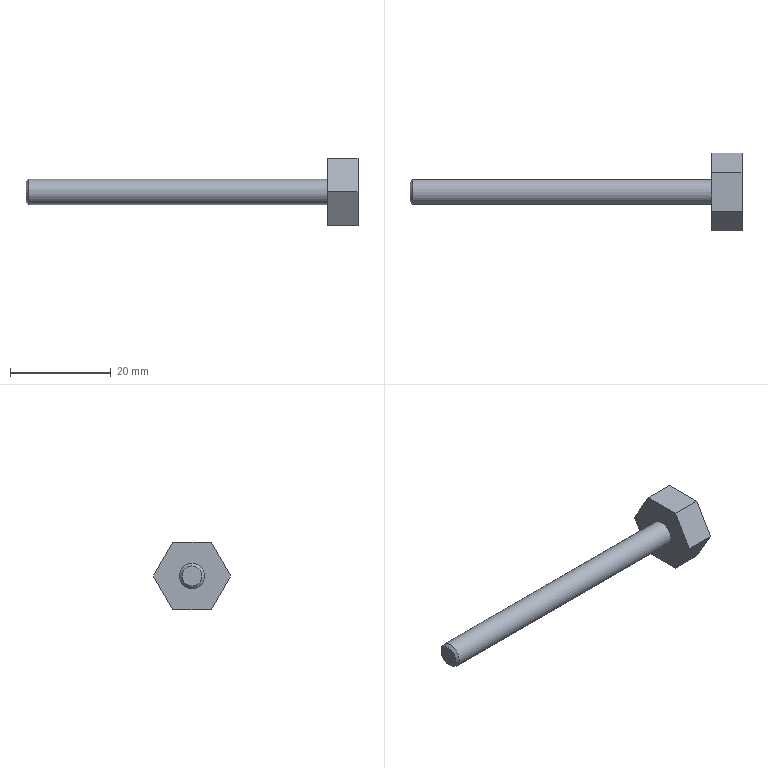Part | NX | features DATUM_CSYS 4, EXTRUDE 3, OFFSET_REGION 3, SKETCH 3, CHAMFER 1 | 1 solid | 18 faces | box 66 x 15.381 x 13.321 mm | volume 1888 mm3 | plane 16 | cylinder 1 | cone 1 | commonest cylinder face diameters 5 x1
STEP:
#1=CARTESIAN_POINT('',(76.,-7.691,0.));
#2=VERTEX_POINT('',#1);
#3=CARTESIAN_POINT('',(76.,-3.845,-6.66));
#4=VERTEX_POINT('',#3);
#5=CARTESIAN_POINT('',(76.,-8.268,1.));
#6=DIRECTION('',(0.,0.5,-0.866));
#7=VECTOR('',#6,1000.);
#8=LINE('',#5,#7);
#9=EDGE_CURVE('',#2,#4,#8,.T.);
#10=ORIENTED_EDGE('',*,*,#9,.T.);
#11=CARTESIAN_POINT('',(76.,3.845,-6.66));
#12=VERTEX_POINT('',#11);
#13=CARTESIAN_POINT('',(76.,-5.,-6.66));
#14=DIRECTION('',(0.,1.,0.));
#15=VECTOR('',#14,1000.);
#16=LINE('',#13,#15);
#17=EDGE_CURVE('',#4,#12,#16,.T.);
#18=ORIENTED_EDGE('',*,*,#17,.T.);
#19=CARTESIAN_POINT('',(76.,7.691,0.));
#20=VERTEX_POINT('',#19);
#21=CARTESIAN_POINT('',(76.,3.268,-7.66));
#22=DIRECTION('',(0.,0.5,0.866));
#23=VECTOR('',#22,1000.);
#24=LINE('',#21,#23);
#25=EDGE_CURVE('',#12,#20,#24,.T.);
#26=ORIENTED_EDGE('',*,*,#25,.T.);
#27=CARTESIAN_POINT('',(76.,3.845,6.66));
#28=VERTEX_POINT('',#27);
#29=CARTESIAN_POINT('',(76.,8.268,-1.));
#30=DIRECTION('',(0.,-0.5,0.866));
#31=VECTOR('',#30,1000.);
#32=LINE('',#29,#31);
#33=EDGE_CURVE('',#20,#28,#32,.T.);
#34=ORIENTED_EDGE('',*,*,#33,.T.);
#35=CARTESIAN_POINT('',(76.,-3.845,6.66));
#36=VERTEX_POINT('',#35);
#37=CARTESIAN_POINT('',(76.,5.,6.66));
#38=DIRECTION('',(0.,-1.,0.));
#39=VECTOR('',#38,1000.);
#40=LINE('',#37,#39);
#41=EDGE_CURVE('',#28,#36,#40,.T.);
#42=ORIENTED_EDGE('',*,*,#41,.T.);
#43=CARTESIAN_POINT('',(76.,-3.268,7.66));
#44=DIRECTION('',(0.,-0.5,-0.866));
#45=VECTOR('',#44,1000.);
#46=LINE('',#43,#45);
#47=EDGE_CURVE('',#36,#2,#46,.T.);
#48=ORIENTED_EDGE('',*,*,#47,.T.);
#49=EDGE_LOOP('',(#10,#18,#26,#34,#42,#48));
#50=FACE_BOUND('',#49,.T.);
#51=CARTESIAN_POINT('',(76.,5.097,-1.008));
#52=VERTEX_POINT('',#51);
#53=CARTESIAN_POINT('',(76.,1.676,-4.918));
#54=VERTEX_POINT('',#53);
#55=CARTESIAN_POINT('',(76.,5.097,-1.008));
#56=DIRECTION('',(0.,-0.6585,-0.7526));
#57=VECTOR('',#56,1000.);
#58=LINE('',#55,#57);
#59=EDGE_CURVE('',#52,#54,#58,.T.);
#60=ORIENTED_EDGE('',*,*,#59,.T.);
#61=CARTESIAN_POINT('',(76.,-3.422,-3.911));
#62=VERTEX_POINT('',#61);
#63=CARTESIAN_POINT('',(76.,1.676,-4.918));
#64=DIRECTION('',(0.,-0.981,0.194));
#65=VECTOR('',#64,1000.);
#66=LINE('',#63,#65);
#67=EDGE_CURVE('',#54,#62,#66,.T.);
#68=ORIENTED_EDGE('',*,*,#67,.T.);
#69=CARTESIAN_POINT('',(76.,-5.097,1.008));
#70=VERTEX_POINT('',#69);
#71=CARTESIAN_POINT('',(76.,-3.422,-3.911));
#72=DIRECTION('',(0.,-0.3225,0.9466));
#73=VECTOR('',#72,1000.);
#74=LINE('',#71,#73);
#75=EDGE_CURVE('',#62,#70,#74,.T.);
#76=ORIENTED_EDGE('',*,*,#75,.T.);
#77=CARTESIAN_POINT('',(76.,-1.676,4.918));
#78=VERTEX_POINT('',#77);
#79=CARTESIAN_POINT('',(76.,-5.097,1.008));
#80=DIRECTION('',(0.,0.6585,0.7526));
#81=VECTOR('',#80,1000.);
#82=LINE('',#79,#81);
#83=EDGE_CURVE('',#70,#78,#82,.T.);
#84=ORIENTED_EDGE('',*,*,#83,.T.);
#85=CARTESIAN_POINT('',(76.,3.422,3.911));
#86=VERTEX_POINT('',#85);
#87=CARTESIAN_POINT('',(76.,-1.676,4.918));
#88=DIRECTION('',(0.,0.981,-0.194));
#89=VECTOR('',#88,1000.);
#90=LINE('',#87,#89);
#91=EDGE_CURVE('',#78,#86,#90,.T.);
#92=ORIENTED_EDGE('',*,*,#91,.T.);
#93=CARTESIAN_POINT('',(76.,3.422,3.911));
#94=DIRECTION('',(0.,0.3225,-0.9466));
#95=VECTOR('',#94,1000.);
#96=LINE('',#93,#95);
#97=EDGE_CURVE('',#86,#52,#96,.T.);
#98=ORIENTED_EDGE('',*,*,#97,.T.);
#99=EDGE_LOOP('',(#60,#68,#76,#84,#92,#98));
#100=FACE_BOUND('',#99,.T.);
#101=CARTESIAN_POINT('',(76.,0.,0.));
#102=DIRECTION('',(1.,0.,0.));
#103=DIRECTION('',(0.,0.,-1.));
#104=AXIS2_PLACEMENT_3D('',#101,#102,#103);
#105=PLANE('',#104);
#106=ADVANCED_FACE('',(#50,#100),#105,.T.);
#107=CARTESIAN_POINT('',(10.5,0.,-2.5));
#108=VERTEX_POINT('',#107);
#109=CARTESIAN_POINT('',(10.5,0.,0.));
#110=DIRECTION('',(1.,0.,0.));
#111=DIRECTION('',(0.,0.,-1.));
#112=AXIS2_PLACEMENT_3D('',#109,#110,#111);
#113=CIRCLE('',#112,2.5);
#114=EDGE_CURVE('',#108,#108,#113,.T.);
#115=ORIENTED_EDGE('',*,*,#114,.T.);
#116=EDGE_LOOP('',(#115));
#117=FACE_BOUND('',#116,.T.);
#118=CARTESIAN_POINT('',(70.,0.,-2.5));
#119=VERTEX_POINT('',#118);
#120=CARTESIAN_POINT('',(70.,0.,0.));
#121=DIRECTION('',(1.,0.,0.));
#122=DIRECTION('',(0.,0.,-1.));
#123=AXIS2_PLACEMENT_3D('',#120,#121,#122);
#124=CIRCLE('',#123,2.5);
#125=EDGE_CURVE('',#119,#119,#124,.T.);
#126=ORIENTED_EDGE('',*,*,#125,.F.);
#127=EDGE_LOOP('',(#126));
#128=FACE_BOUND('',#127,.T.);
#129=CARTESIAN_POINT('',(70.,0.,0.));
#130=DIRECTION('',(-1.,0.,0.));
#131=DIRECTION('',(0.,0.,1.));
#132=AXIS2_PLACEMENT_3D('',#129,#130,#131);
#133=CYLINDRICAL_SURFACE('',#132,2.5);
#134=ADVANCED_FACE('',(#117,#128),#133,.T.);
#135=CARTESIAN_POINT('',(10.,0.,-2.));
#136=VERTEX_POINT('',#135);
#137=CARTESIAN_POINT('',(10.,0.,0.));
#138=DIRECTION('',(1.,0.,0.));
#139=DIRECTION('',(0.,0.,-1.));
#140=AXIS2_PLACEMENT_3D('',#137,#138,#139);
#141=CIRCLE('',#140,2.);
#142=EDGE_CURVE('',#136,#136,#141,.F.);
#143=ORIENTED_EDGE('',*,*,#142,.T.);
#144=EDGE_LOOP('',(#143));
#145=FACE_BOUND('',#144,.T.);
#146=CARTESIAN_POINT('',(10.,0.,0.));
#147=DIRECTION('',(1.,0.,0.));
#148=DIRECTION('',(0.,0.,-1.));
#149=AXIS2_PLACEMENT_3D('',#146,#147,#148);
#150=PLANE('',#149);
#151=ADVANCED_FACE('',(#145),#150,.F.);
#152=CARTESIAN_POINT('',(70.,-7.691,0.));
#153=VERTEX_POINT('',#152);
#154=CARTESIAN_POINT('',(70.,-3.845,-6.66));
#155=VERTEX_POINT('',#154);
#156=CARTESIAN_POINT('',(70.,-8.268,1.));
#157=DIRECTION('',(0.,0.5,-0.866));
#158=VECTOR('',#157,1000.);
#159=LINE('',#156,#158);
#160=EDGE_CURVE('',#153,#155,#159,.T.);
#161=ORIENTED_EDGE('',*,*,#160,.T.);
#162=CARTESIAN_POINT('',(76.,-3.845,-6.66));
#163=DIRECTION('',(-1.,0.,0.));
#164=VECTOR('',#163,1000.);
#165=LINE('',#162,#164);
#166=EDGE_CURVE('',#4,#155,#165,.T.);
#167=ORIENTED_EDGE('',*,*,#166,.F.);
#168=ORIENTED_EDGE('',*,*,#9,.F.);
#169=CARTESIAN_POINT('',(76.,-7.691,0.));
#170=DIRECTION('',(-1.,0.,0.));
#171=VECTOR('',#170,1000.);
#172=LINE('',#169,#171);
#173=EDGE_CURVE('',#2,#153,#172,.T.);
#174=ORIENTED_EDGE('',*,*,#173,.T.);
#175=EDGE_LOOP('',(#161,#167,#168,#174));
#176=FACE_BOUND('',#175,.T.);
#177=CARTESIAN_POINT('',(76.,-8.268,1.));
#178=DIRECTION('',(0.,0.866,0.5));
#179=DIRECTION('',(0.,-0.5,0.866));
#180=AXIS2_PLACEMENT_3D('',#177,#178,#179);
#181=PLANE('',#180);
#182=ADVANCED_FACE('',(#176),#181,.F.);
#183=CARTESIAN_POINT('',(70.,3.845,-6.66));
#184=VERTEX_POINT('',#183);
#185=CARTESIAN_POINT('',(70.,-5.,-6.66));
#186=DIRECTION('',(0.,1.,0.));
#187=VECTOR('',#186,1000.);
#188=LINE('',#185,#187);
#189=EDGE_CURVE('',#155,#184,#188,.T.);
#190=ORIENTED_EDGE('',*,*,#189,.T.);
#191=CARTESIAN_POINT('',(76.,3.845,-6.66));
#192=DIRECTION('',(-1.,0.,0.));
#193=VECTOR('',#192,1000.);
#194=LINE('',#191,#193);
#195=EDGE_CURVE('',#12,#184,#194,.T.);
#196=ORIENTED_EDGE('',*,*,#195,.F.);
#197=ORIENTED_EDGE('',*,*,#17,.F.);
#198=ORIENTED_EDGE('',*,*,#166,.T.);
#199=EDGE_LOOP('',(#190,#196,#197,#198));
#200=FACE_BOUND('',#199,.T.);
#201=CARTESIAN_POINT('',(76.,-5.,-6.66));
#202=DIRECTION('',(0.,0.,1.));
#203=DIRECTION('',(0.,-1.,0.));
#204=AXIS2_PLACEMENT_3D('',#201,#202,#203);
#205=PLANE('',#204);
#206=ADVANCED_FACE('',(#200),#205,.F.);
#207=CARTESIAN_POINT('',(70.,7.691,0.));
#208=VERTEX_POINT('',#207);
#209=CARTESIAN_POINT('',(70.,3.268,-7.66));
#210=DIRECTION('',(0.,0.5,0.866));
#211=VECTOR('',#210,1000.);
#212=LINE('',#209,#211);
#213=EDGE_CURVE('',#184,#208,#212,.T.);
#214=ORIENTED_EDGE('',*,*,#213,.T.);
#215=CARTESIAN_POINT('',(76.,7.691,0.));
#216=DIRECTION('',(-1.,0.,0.));
#217=VECTOR('',#216,1000.);
#218=LINE('',#215,#217);
#219=EDGE_CURVE('',#20,#208,#218,.T.);
#220=ORIENTED_EDGE('',*,*,#219,.F.);
#221=ORIENTED_EDGE('',*,*,#25,.F.);
#222=ORIENTED_EDGE('',*,*,#195,.T.);
#223=EDGE_LOOP('',(#214,#220,#221,#222));
#224=FACE_BOUND('',#223,.T.);
#225=CARTESIAN_POINT('',(76.,3.268,-7.66));
#226=DIRECTION('',(0.,-0.866,0.5));
#227=DIRECTION('',(0.,-0.5,-0.866));
#228=AXIS2_PLACEMENT_3D('',#225,#226,#227);
#229=PLANE('',#228);
#230=ADVANCED_FACE('',(#224),#229,.F.);
#231=CARTESIAN_POINT('',(70.,3.845,6.66));
#232=VERTEX_POINT('',#231);
#233=CARTESIAN_POINT('',(70.,8.268,-1.));
#234=DIRECTION('',(0.,-0.5,0.866));
#235=VECTOR('',#234,1000.);
#236=LINE('',#233,#235);
#237=EDGE_CURVE('',#208,#232,#236,.T.);
#238=ORIENTED_EDGE('',*,*,#237,.T.);
#239=CARTESIAN_POINT('',(76.,3.845,6.66));
#240=DIRECTION('',(-1.,0.,0.));
#241=VECTOR('',#240,1000.);
#242=LINE('',#239,#241);
#243=EDGE_CURVE('',#28,#232,#242,.T.);
#244=ORIENTED_EDGE('',*,*,#243,.F.);
#245=ORIENTED_EDGE('',*,*,#33,.F.);
#246=ORIENTED_EDGE('',*,*,#219,.T.);
#247=EDGE_LOOP('',(#238,#244,#245,#246));
#248=FACE_BOUND('',#247,.T.);
#249=CARTESIAN_POINT('',(76.,8.268,-1.));
#250=DIRECTION('',(0.,-0.866,-0.5));
#251=DIRECTION('',(0.,0.5,-0.866));
#252=AXIS2_PLACEMENT_3D('',#249,#250,#251);
#253=PLANE('',#252);
#254=ADVANCED_FACE('',(#248),#253,.F.);
#255=CARTESIAN_POINT('',(70.,-3.845,6.66));
#256=VERTEX_POINT('',#255);
#257=CARTESIAN_POINT('',(70.,5.,6.66));
#258=DIRECTION('',(0.,-1.,0.));
#259=VECTOR('',#258,1000.);
#260=LINE('',#257,#259);
#261=EDGE_CURVE('',#232,#256,#260,.T.);
#262=ORIENTED_EDGE('',*,*,#261,.T.);
#263=CARTESIAN_POINT('',(76.,-3.845,6.66));
#264=DIRECTION('',(-1.,0.,0.));
#265=VECTOR('',#264,1000.);
#266=LINE('',#263,#265);
#267=EDGE_CURVE('',#36,#256,#266,.T.);
#268=ORIENTED_EDGE('',*,*,#267,.F.);
#269=ORIENTED_EDGE('',*,*,#41,.F.);
#270=ORIENTED_EDGE('',*,*,#243,.T.);
#271=EDGE_LOOP('',(#262,#268,#269,#270));
#272=FACE_BOUND('',#271,.T.);
#273=CARTESIAN_POINT('',(76.,5.,6.66));
#274=DIRECTION('',(0.,0.,-1.));
#275=DIRECTION('',(0.,1.,0.));
#276=AXIS2_PLACEMENT_3D('',#273,#274,#275);
#277=PLANE('',#276);
#278=ADVANCED_FACE('',(#272),#277,.F.);
#279=CARTESIAN_POINT('',(70.,-3.268,7.66));
#280=DIRECTION('',(0.,-0.5,-0.866));
#281=VECTOR('',#280,1000.);
#282=LINE('',#279,#281);
#283=EDGE_CURVE('',#256,#153,#282,.T.);
#284=ORIENTED_EDGE('',*,*,#283,.T.);
#285=ORIENTED_EDGE('',*,*,#173,.F.);
#286=ORIENTED_EDGE('',*,*,#47,.F.);
#287=ORIENTED_EDGE('',*,*,#267,.T.);
#288=EDGE_LOOP('',(#284,#285,#286,#287));
#289=FACE_BOUND('',#288,.T.);
#290=CARTESIAN_POINT('',(76.,-3.268,7.66));
#291=DIRECTION('',(0.,0.866,-0.5));
#292=DIRECTION('',(0.,0.5,0.866));
#293=AXIS2_PLACEMENT_3D('',#290,#291,#292);
#294=PLANE('',#293);
#295=ADVANCED_FACE('',(#289),#294,.F.);
#296=ORIENTED_EDGE('',*,*,#125,.T.);
#297=EDGE_LOOP('',(#296));
#298=FACE_BOUND('',#297,.T.);
#299=ORIENTED_EDGE('',*,*,#160,.F.);
#300=ORIENTED_EDGE('',*,*,#283,.F.);
#301=ORIENTED_EDGE('',*,*,#261,.F.);
#302=ORIENTED_EDGE('',*,*,#237,.F.);
#303=ORIENTED_EDGE('',*,*,#213,.F.);
#304=ORIENTED_EDGE('',*,*,#189,.F.);
#305=EDGE_LOOP('',(#299,#300,#301,#302,#303,#304));
#306=FACE_BOUND('',#305,.T.);
#307=CARTESIAN_POINT('',(70.,0.,0.));
#308=DIRECTION('',(1.,0.,0.));
#309=DIRECTION('',(0.,0.,-1.));
#310=AXIS2_PLACEMENT_3D('',#307,#308,#309);
#311=PLANE('',#310);
#312=ADVANCED_FACE('',(#298,#306),#311,.F.);
#313=ORIENTED_EDGE('',*,*,#142,.F.);
#314=EDGE_LOOP('',(#313));
#315=FACE_BOUND('',#314,.T.);
#316=ORIENTED_EDGE('',*,*,#114,.F.);
#317=EDGE_LOOP('',(#316));
#318=FACE_BOUND('',#317,.T.);
#319=CARTESIAN_POINT('',(10.5,0.,0.));
#320=DIRECTION('',(1.,0.,0.));
#321=DIRECTION('',(0.,0.,-1.));
#322=AXIS2_PLACEMENT_3D('',#319,#320,#321);
#323=CONICAL_SURFACE('',#322,2.5,0.7854);
#324=ADVANCED_FACE('',(#315,#318),#323,.T.);
#325=ORIENTED_EDGE('',*,*,#67,.F.);
#326=CARTESIAN_POINT('',(73.,1.676,-4.918));
#327=VERTEX_POINT('',#326);
#328=CARTESIAN_POINT('',(73.,1.676,-4.918));
#329=DIRECTION('',(1.,0.,0.));
#330=VECTOR('',#329,1000.);
#331=LINE('',#328,#330);
#332=EDGE_CURVE('',#54,#327,#331,.F.);
#333=ORIENTED_EDGE('',*,*,#332,.T.);
#334=CARTESIAN_POINT('',(73.,-3.422,-3.911));
#335=VERTEX_POINT('',#334);
#336=CARTESIAN_POINT('',(73.,1.676,-4.918));
#337=DIRECTION('',(0.,-0.981,0.194));
#338=VECTOR('',#337,1000.);
#339=LINE('',#336,#338);
#340=EDGE_CURVE('',#335,#327,#339,.F.);
#341=ORIENTED_EDGE('',*,*,#340,.F.);
#342=CARTESIAN_POINT('',(73.,-3.422,-3.911));
#343=DIRECTION('',(1.,0.,0.));
#344=VECTOR('',#343,1000.);
#345=LINE('',#342,#344);
#346=EDGE_CURVE('',#62,#335,#345,.F.);
#347=ORIENTED_EDGE('',*,*,#346,.F.);
#348=EDGE_LOOP('',(#325,#333,#341,#347));
#349=FACE_BOUND('',#348,.T.);
#350=CARTESIAN_POINT('',(73.,1.676,-4.918));
#351=DIRECTION('',(0.,0.194,0.981));
#352=DIRECTION('',(0.,-0.981,0.194));
#353=AXIS2_PLACEMENT_3D('',#350,#351,#352);
#354=PLANE('',#353);
#355=ADVANCED_FACE('',(#349),#354,.T.);
#356=ORIENTED_EDGE('',*,*,#75,.F.);
#357=ORIENTED_EDGE('',*,*,#346,.T.);
#358=CARTESIAN_POINT('',(73.,-5.097,1.008));
#359=VERTEX_POINT('',#358);
#360=CARTESIAN_POINT('',(73.,-3.422,-3.911));
#361=DIRECTION('',(0.,-0.3225,0.9466));
#362=VECTOR('',#361,1000.);
#363=LINE('',#360,#362);
#364=EDGE_CURVE('',#359,#335,#363,.F.);
#365=ORIENTED_EDGE('',*,*,#364,.F.);
#366=CARTESIAN_POINT('',(73.,-5.097,1.008));
#367=DIRECTION('',(1.,0.,0.));
#368=VECTOR('',#367,1000.);
#369=LINE('',#366,#368);
#370=EDGE_CURVE('',#70,#359,#369,.F.);
#371=ORIENTED_EDGE('',*,*,#370,.F.);
#372=EDGE_LOOP('',(#356,#357,#365,#371));
#373=FACE_BOUND('',#372,.T.);
#374=CARTESIAN_POINT('',(73.,-3.422,-3.911));
#375=DIRECTION('',(0.,0.9466,0.3225));
#376=DIRECTION('',(0.,-0.3225,0.9466));
#377=AXIS2_PLACEMENT_3D('',#374,#375,#376);
#378=PLANE('',#377);
#379=ADVANCED_FACE('',(#373),#378,.T.);
#380=ORIENTED_EDGE('',*,*,#83,.F.);
#381=ORIENTED_EDGE('',*,*,#370,.T.);
#382=CARTESIAN_POINT('',(73.,-1.676,4.918));
#383=VERTEX_POINT('',#382);
#384=CARTESIAN_POINT('',(73.,-5.097,1.008));
#385=DIRECTION('',(0.,0.6585,0.7526));
#386=VECTOR('',#385,1000.);
#387=LINE('',#384,#386);
#388=EDGE_CURVE('',#383,#359,#387,.F.);
#389=ORIENTED_EDGE('',*,*,#388,.F.);
#390=CARTESIAN_POINT('',(73.,-1.676,4.918));
#391=DIRECTION('',(1.,0.,0.));
#392=VECTOR('',#391,1000.);
#393=LINE('',#390,#392);
#394=EDGE_CURVE('',#78,#383,#393,.F.);
#395=ORIENTED_EDGE('',*,*,#394,.F.);
#396=EDGE_LOOP('',(#380,#381,#389,#395));
#397=FACE_BOUND('',#396,.T.);
#398=CARTESIAN_POINT('',(73.,-5.097,1.008));
#399=DIRECTION('',(0.,0.7526,-0.6585));
#400=DIRECTION('',(0.,0.6585,0.7526));
#401=AXIS2_PLACEMENT_3D('',#398,#399,#400);
#402=PLANE('',#401);
#403=ADVANCED_FACE('',(#397),#402,.T.);
#404=ORIENTED_EDGE('',*,*,#91,.F.);
#405=ORIENTED_EDGE('',*,*,#394,.T.);
#406=CARTESIAN_POINT('',(73.,3.422,3.911));
#407=VERTEX_POINT('',#406);
#408=CARTESIAN_POINT('',(73.,-1.676,4.918));
#409=DIRECTION('',(0.,0.981,-0.194));
#410=VECTOR('',#409,1000.);
#411=LINE('',#408,#410);
#412=EDGE_CURVE('',#407,#383,#411,.F.);
#413=ORIENTED_EDGE('',*,*,#412,.F.);
#414=CARTESIAN_POINT('',(73.,3.422,3.911));
#415=DIRECTION('',(1.,0.,0.));
#416=VECTOR('',#415,1000.);
#417=LINE('',#414,#416);
#418=EDGE_CURVE('',#86,#407,#417,.F.);
#419=ORIENTED_EDGE('',*,*,#418,.F.);
#420=EDGE_LOOP('',(#404,#405,#413,#419));
#421=FACE_BOUND('',#420,.T.);
#422=CARTESIAN_POINT('',(73.,-1.676,4.918));
#423=DIRECTION('',(0.,-0.194,-0.981));
#424=DIRECTION('',(0.,0.981,-0.194));
#425=AXIS2_PLACEMENT_3D('',#422,#423,#424);
#426=PLANE('',#425);
#427=ADVANCED_FACE('',(#421),#426,.T.);
#428=ORIENTED_EDGE('',*,*,#97,.F.);
#429=ORIENTED_EDGE('',*,*,#418,.T.);
#430=CARTESIAN_POINT('',(73.,5.097,-1.008));
#431=VERTEX_POINT('',#430);
#432=CARTESIAN_POINT('',(73.,3.422,3.911));
#433=DIRECTION('',(0.,0.3225,-0.9466));
#434=VECTOR('',#433,1000.);
#435=LINE('',#432,#434);
#436=EDGE_CURVE('',#431,#407,#435,.F.);
#437=ORIENTED_EDGE('',*,*,#436,.F.);
#438=CARTESIAN_POINT('',(73.,5.097,-1.008));
#439=DIRECTION('',(1.,0.,0.));
#440=VECTOR('',#439,1000.);
#441=LINE('',#438,#440);
#442=EDGE_CURVE('',#52,#431,#441,.F.);
#443=ORIENTED_EDGE('',*,*,#442,.F.);
#444=EDGE_LOOP('',(#428,#429,#437,#443));
#445=FACE_BOUND('',#444,.T.);
#446=CARTESIAN_POINT('',(73.,3.422,3.911));
#447=DIRECTION('',(0.,-0.9466,-0.3225));
#448=DIRECTION('',(0.,0.3225,-0.9466));
#449=AXIS2_PLACEMENT_3D('',#446,#447,#448);
#450=PLANE('',#449);
#451=ADVANCED_FACE('',(#445),#450,.T.);
#452=ORIENTED_EDGE('',*,*,#59,.F.);
#453=ORIENTED_EDGE('',*,*,#442,.T.);
#454=CARTESIAN_POINT('',(73.,5.097,-1.008));
#455=DIRECTION('',(0.,-0.6585,-0.7526));
#456=VECTOR('',#455,1000.);
#457=LINE('',#454,#456);
#458=EDGE_CURVE('',#327,#431,#457,.F.);
#459=ORIENTED_EDGE('',*,*,#458,.F.);
#460=ORIENTED_EDGE('',*,*,#332,.F.);
#461=EDGE_LOOP('',(#452,#453,#459,#460));
#462=FACE_BOUND('',#461,.T.);
#463=CARTESIAN_POINT('',(73.,5.097,-1.008));
#464=DIRECTION('',(0.,-0.7526,0.6585));
#465=DIRECTION('',(0.,-0.6585,-0.7526));
#466=AXIS2_PLACEMENT_3D('',#463,#464,#465);
#467=PLANE('',#466);
#468=ADVANCED_FACE('',(#462),#467,.T.);
#469=ORIENTED_EDGE('',*,*,#340,.T.);
#470=ORIENTED_EDGE('',*,*,#458,.T.);
#471=ORIENTED_EDGE('',*,*,#436,.T.);
#472=ORIENTED_EDGE('',*,*,#412,.T.);
#473=ORIENTED_EDGE('',*,*,#388,.T.);
#474=ORIENTED_EDGE('',*,*,#364,.T.);
#475=EDGE_LOOP('',(#469,#470,#471,#472,#473,#474));
#476=FACE_BOUND('',#475,.T.);
#477=CARTESIAN_POINT('',(73.,0.,0.));
#478=DIRECTION('',(-1.,0.,0.));
#479=DIRECTION('',(0.,0.,1.));
#480=AXIS2_PLACEMENT_3D('',#477,#478,#479);
#481=PLANE('',#480);
#482=ADVANCED_FACE('',(#476),#481,.F.);
#483=CLOSED_SHELL('',(#106,#134,#151,#182,#206,#230,#254,#278,#295,#312,#324,#355,#379,#403,#427,#451,#468,#482));
#484=MANIFOLD_SOLID_BREP('',#483);
#485=(LENGTH_UNIT()NAMED_UNIT(*)SI_UNIT(.MILLI.,.METRE.));
#486=UNCERTAINTY_MEASURE_WITH_UNIT(LENGTH_MEASURE(0.00001),#485,'','');
#487=(NAMED_UNIT(*)PLANE_ANGLE_UNIT()SI_UNIT($,.RADIAN.));
#488=(NAMED_UNIT(*)SI_UNIT($,.STERADIAN.)SOLID_ANGLE_UNIT());
#489=(GEOMETRIC_REPRESENTATION_CONTEXT(3)GLOBAL_UNCERTAINTY_ASSIGNED_CONTEXT((#486))GLOBAL_UNIT_ASSIGNED_CONTEXT((#485,#487,#488))REPRESENTATION_CONTEXT('',''));
#490=ADVANCED_BREP_SHAPE_REPRESENTATION('',(#484),#489);